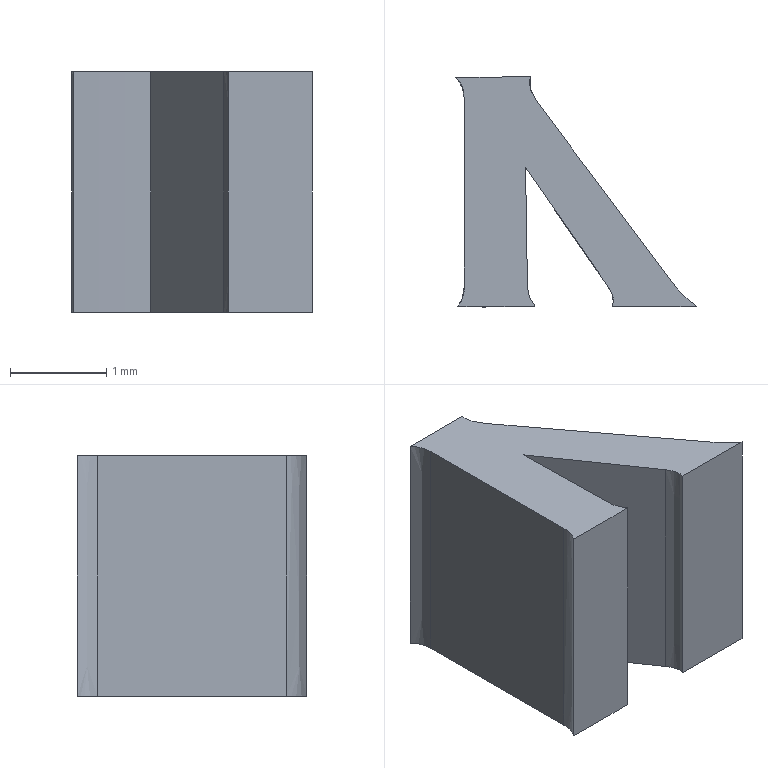Part | STEP file | lll_id1114_x_t | 1 solid | 15 faces | box 2.507 x 2.385 x 2.5 mm | volume 6.979 mm3 | plane 8 | other 4 | cylinder 3 | commonest cylinder face diameters 0.673 x1 2.106 x1 55.706 x1
STEP:
#1=CARTESIAN_POINT('',(392.49,-124.732,2.35));
#2=VERTEX_POINT('',#1);
#3=CARTESIAN_POINT('',(392.719,-124.959,2.35));
#4=VERTEX_POINT('',#3);
#5=CARTESIAN_POINT('',(393.33,-124.099,2.35));
#6=DIRECTION('',(0.,0.,1.));
#7=DIRECTION('',(-1.,0.,0.));
#8=AXIS2_PLACEMENT_3D('',#5,#6,#7);
#9=CIRCLE('',#8,1.053);
#10=EDGE_CURVE('',#2,#4,#9,.T.);
#11=ORIENTED_EDGE('',*,*,#10,.T.);
#12=CARTESIAN_POINT('',(392.719,-124.959,-0.15));
#13=VERTEX_POINT('',#12);
#14=CARTESIAN_POINT('',(392.727,-124.962,-0.15));
#15=DIRECTION('',(0.,0.,1.));
#16=VECTOR('',#15,1.);
#17=LINE('',#14,#16);
#18=EDGE_CURVE('',#13,#4,#17,.T.);
#19=ORIENTED_EDGE('',*,*,#18,.F.);
#20=CARTESIAN_POINT('',(392.49,-124.732,-0.15));
#21=VERTEX_POINT('',#20);
#22=CARTESIAN_POINT('',(393.33,-124.099,-0.15));
#23=DIRECTION('',(0.,0.,1.));
#24=DIRECTION('',(-1.,0.,0.));
#25=AXIS2_PLACEMENT_3D('',#22,#23,#24);
#26=CIRCLE('',#25,1.053);
#27=EDGE_CURVE('',#21,#13,#26,.T.);
#28=ORIENTED_EDGE('',*,*,#27,.F.);
#29=CARTESIAN_POINT('',(392.49,-124.732,-0.15));
#30=DIRECTION('',(0.,0.,1.));
#31=VECTOR('',#30,1.);
#32=LINE('',#29,#31);
#33=EDGE_CURVE('',#21,#2,#32,.T.);
#34=ORIENTED_EDGE('',*,*,#33,.T.);
#35=EDGE_LOOP('',(#11,#19,#28,#34));
#36=FACE_OUTER_BOUND('',#35,.T.);
#37=CARTESIAN_POINT('',(393.33,-124.099,-0.15));
#38=DIRECTION('',(0.,0.,1.));
#39=DIRECTION('',(1.,0.,0.));
#40=AXIS2_PLACEMENT_3D('',#37,#38,#39);
#41=CYLINDRICAL_SURFACE('',#40,1.053);
#42=ADVANCED_FACE('',(#36),#41,.F.);
#43=CARTESIAN_POINT('',(391.85,-124.96,2.35));
#44=VERTEX_POINT('',#43);
#45=CARTESIAN_POINT('',(392.719,-124.962,2.35));
#46=DIRECTION('',(-1.,0.,0.));
#47=VECTOR('',#46,1.);
#48=LINE('',#45,#47);
#49=EDGE_CURVE('',#4,#44,#48,.T.);
#50=ORIENTED_EDGE('',*,*,#49,.T.);
#51=CARTESIAN_POINT('',(391.85,-124.96,-0.15));
#52=VERTEX_POINT('',#51);
#53=CARTESIAN_POINT('',(391.849,-124.962,-0.15));
#54=DIRECTION('',(0.,0.,1.));
#55=VECTOR('',#54,1.);
#56=LINE('',#53,#55);
#57=EDGE_CURVE('',#52,#44,#56,.T.);
#58=ORIENTED_EDGE('',*,*,#57,.F.);
#59=CARTESIAN_POINT('',(392.719,-124.962,-0.15));
#60=DIRECTION('',(-1.,0.,0.));
#61=VECTOR('',#60,1.);
#62=LINE('',#59,#61);
#63=EDGE_CURVE('',#13,#52,#62,.T.);
#64=ORIENTED_EDGE('',*,*,#63,.F.);
#65=ORIENTED_EDGE('',*,*,#18,.T.);
#66=EDGE_LOOP('',(#50,#58,#64,#65));
#67=FACE_OUTER_BOUND('',#66,.T.);
#68=CARTESIAN_POINT('',(392.719,-124.962,-0.15));
#69=DIRECTION('',(0.,1.,0.));
#70=DIRECTION('',(0.,0.,1.));
#71=AXIS2_PLACEMENT_3D('',#68,#69,#70);
#72=PLANE('',#71);
#73=ADVANCED_FACE('',(#67),#72,.F.);
#74=CARTESIAN_POINT('',(391.803,-124.75,2.35));
#75=VERTEX_POINT('',#74);
#76=CARTESIAN_POINT('',(391.85,-124.958,2.35));
#77=CARTESIAN_POINT('',(391.856,-124.941,2.35));
#78=CARTESIAN_POINT('',(391.859,-124.924,2.35));
#79=CARTESIAN_POINT('',(391.86,-124.892,2.35));
#80=CARTESIAN_POINT('',(391.859,-124.877,2.35));
#81=CARTESIAN_POINT('',(391.854,-124.853,2.35));
#82=CARTESIAN_POINT('',(391.851,-124.844,2.35));
#83=CARTESIAN_POINT('',(391.844,-124.824,2.35));
#84=CARTESIAN_POINT('',(391.84,-124.814,2.35));
#85=CARTESIAN_POINT('',(391.827,-124.789,2.35));
#86=CARTESIAN_POINT('',(391.819,-124.775,2.35));
#87=CARTESIAN_POINT('',(391.808,-124.757,2.35));
#88=CARTESIAN_POINT('',(391.805,-124.753,2.35));
#89=CARTESIAN_POINT('',(391.803,-124.75,2.35));
#90=(BOUNDED_CURVE()B_SPLINE_CURVE(3,(#76,#77,#78,#79,#80,#81,#82,#83,#84,#85,#86,#87,#88,#89),.UNSPECIFIED.,.F.,.F.)B_SPLINE_CURVE_WITH_KNOTS((4,2,2,2,2,2,4),(0.,0.2364,0.4388,0.5636,0.7197,0.9376,1.),.UNSPECIFIED.)CURVE()GEOMETRIC_REPRESENTATION_ITEM()RATIONAL_B_SPLINE_CURVE((0.502,0.4993,0.4993,0.499,0.499,0.5013,0.5013,0.5014,0.5014,0.5014,0.5014,0.502,0.502,0.502))REPRESENTATION_ITEM(''));
#91=EDGE_CURVE('',#44,#75,#90,.T.);
#92=ORIENTED_EDGE('',*,*,#91,.T.);
#93=CARTESIAN_POINT('',(391.803,-124.75,-0.15));
#94=VERTEX_POINT('',#93);
#95=CARTESIAN_POINT('',(391.803,-124.75,-0.15));
#96=DIRECTION('',(0.,0.,1.));
#97=VECTOR('',#96,1.);
#98=LINE('',#95,#97);
#99=EDGE_CURVE('',#94,#75,#98,.T.);
#100=ORIENTED_EDGE('',*,*,#99,.F.);
#101=CARTESIAN_POINT('',(391.85,-124.96,-0.15));
#102=CARTESIAN_POINT('',(391.85,-124.959,-0.15));
#103=CARTESIAN_POINT('',(391.85,-124.958,-0.15));
#104=CARTESIAN_POINT('',(391.856,-124.941,-0.15));
#105=CARTESIAN_POINT('',(391.859,-124.924,-0.15));
#106=CARTESIAN_POINT('',(391.86,-124.892,-0.15));
#107=CARTESIAN_POINT('',(391.859,-124.877,-0.15));
#108=CARTESIAN_POINT('',(391.854,-124.853,-0.15));
#109=CARTESIAN_POINT('',(391.851,-124.844,-0.15));
#110=CARTESIAN_POINT('',(391.844,-124.824,-0.15));
#111=CARTESIAN_POINT('',(391.84,-124.814,-0.15));
#112=CARTESIAN_POINT('',(391.827,-124.789,-0.15));
#113=CARTESIAN_POINT('',(391.819,-124.775,-0.15));
#114=CARTESIAN_POINT('',(391.808,-124.757,-0.15));
#115=CARTESIAN_POINT('',(391.805,-124.753,-0.15));
#116=CARTESIAN_POINT('',(391.803,-124.75,-0.15));
#117=(BOUNDED_CURVE()B_SPLINE_CURVE(3,(#101,#102,#103,#104,#105,#106,#107,#108,#109,#110,#111,#112,#113,#114,#115,#116),.UNSPECIFIED.,.F.,.F.)B_SPLINE_CURVE_WITH_KNOTS((4,2,2,2,2,2,2,4),(0.,0.009901,0.2439,0.4443,0.5679,0.7225,0.9382,1.),.UNSPECIFIED.)CURVE()GEOMETRIC_REPRESENTATION_ITEM()RATIONAL_B_SPLINE_CURVE((0.502,0.502,0.502,0.4993,0.4993,0.499,0.499,0.5013,0.5013,0.5014,0.5014,0.5014,0.5014,0.502,0.502,0.502))REPRESENTATION_ITEM(''));
#118=EDGE_CURVE('',#52,#94,#117,.T.);
#119=ORIENTED_EDGE('',*,*,#118,.F.);
#120=ORIENTED_EDGE('',*,*,#57,.T.);
#121=EDGE_LOOP('',(#92,#100,#119,#120));
#122=FACE_OUTER_BOUND('',#121,.T.);
#123=CARTESIAN_POINT('',(391.849,-124.962,-0.15));
#124=CARTESIAN_POINT('',(391.849,-124.961,-0.15));
#125=CARTESIAN_POINT('',(391.849,-124.96,-0.15));
#126=CARTESIAN_POINT('',(391.85,-124.959,-0.15));
#127=CARTESIAN_POINT('',(391.85,-124.958,-0.15));
#128=CARTESIAN_POINT('',(391.856,-124.941,-0.15));
#129=CARTESIAN_POINT('',(391.859,-124.924,-0.15));
#130=CARTESIAN_POINT('',(391.86,-124.892,-0.15));
#131=CARTESIAN_POINT('',(391.859,-124.877,-0.15));
#132=CARTESIAN_POINT('',(391.854,-124.853,-0.15));
#133=CARTESIAN_POINT('',(391.851,-124.844,-0.15));
#134=CARTESIAN_POINT('',(391.844,-124.824,-0.15));
#135=CARTESIAN_POINT('',(391.84,-124.814,-0.15));
#136=CARTESIAN_POINT('',(391.827,-124.789,-0.15));
#137=CARTESIAN_POINT('',(391.819,-124.775,-0.15));
#138=CARTESIAN_POINT('',(391.808,-124.757,-0.15));
#139=CARTESIAN_POINT('',(391.805,-124.753,-0.15));
#140=CARTESIAN_POINT('',(391.803,-124.75,-0.15));
#141=(BOUNDED_CURVE()B_SPLINE_CURVE(3,(#123,#124,#125,#126,#127,#128,#129,#130,#131,#132,#133,#134,#135,#136,#137,#138,#139,#140),.UNSPECIFIED.,.F.,.F.)B_SPLINE_CURVE_WITH_KNOTS((4,2,2,2,2,2,2,2,4),(0.,0.009901,0.0197,0.2514,0.4498,0.5722,0.7252,0.9388,1.),.UNSPECIFIED.)CURVE()GEOMETRIC_REPRESENTATION_ITEM()RATIONAL_B_SPLINE_CURVE((0.502,0.502,0.502,0.502,0.502,0.4993,0.4993,0.499,0.499,0.5013,0.5013,0.5014,0.5014,0.5014,0.5014,0.502,0.502,0.502))REPRESENTATION_ITEM(''));
#142=DIRECTION('',(0.,0.,1.));
#143=VECTOR('',#142,1.);
#144=SURFACE_OF_LINEAR_EXTRUSION('',#141,#143);
#145=ADVANCED_FACE('',(#122),#144,.F.);
#146=CARTESIAN_POINT('',(390.949,-123.517,2.35));
#147=VERTEX_POINT('',#146);
#148=CARTESIAN_POINT('',(391.803,-124.75,2.35));
#149=DIRECTION('',(-0.5693,0.8221,0.));
#150=VECTOR('',#149,1.);
#151=LINE('',#148,#150);
#152=EDGE_CURVE('',#75,#147,#151,.T.);
#153=ORIENTED_EDGE('',*,*,#152,.T.);
#154=CARTESIAN_POINT('',(390.949,-123.517,-0.15));
#155=VERTEX_POINT('',#154);
#156=CARTESIAN_POINT('',(390.949,-123.517,-0.15));
#157=DIRECTION('',(0.,0.,1.));
#158=VECTOR('',#157,1.);
#159=LINE('',#156,#158);
#160=EDGE_CURVE('',#155,#147,#159,.T.);
#161=ORIENTED_EDGE('',*,*,#160,.F.);
#162=CARTESIAN_POINT('',(391.803,-124.75,-0.15));
#163=DIRECTION('',(-0.5693,0.8221,0.));
#164=VECTOR('',#163,1.);
#165=LINE('',#162,#164);
#166=EDGE_CURVE('',#94,#155,#165,.T.);
#167=ORIENTED_EDGE('',*,*,#166,.F.);
#168=ORIENTED_EDGE('',*,*,#99,.T.);
#169=EDGE_LOOP('',(#153,#161,#167,#168));
#170=FACE_OUTER_BOUND('',#169,.T.);
#171=CARTESIAN_POINT('',(391.803,-124.75,-0.15));
#172=DIRECTION('',(0.8221,0.5693,0.));
#173=DIRECTION('',(0.5693,-0.8221,0.));
#174=AXIS2_PLACEMENT_3D('',#171,#172,#173);
#175=PLANE('',#174);
#176=ADVANCED_FACE('',(#170),#175,.F.);
#177=CARTESIAN_POINT('',(390.968,-124.746,2.35));
#178=VERTEX_POINT('',#177);
#179=CARTESIAN_POINT('',(390.949,-123.517,2.35));
#180=DIRECTION('',(0.01539,-0.9999,0.));
#181=VECTOR('',#180,1.);
#182=LINE('',#179,#181);
#183=EDGE_CURVE('',#147,#178,#182,.T.);
#184=ORIENTED_EDGE('',*,*,#183,.T.);
#185=CARTESIAN_POINT('',(390.968,-124.746,-0.15));
#186=VERTEX_POINT('',#185);
#187=CARTESIAN_POINT('',(390.968,-124.746,-0.15));
#188=DIRECTION('',(0.,0.,1.));
#189=VECTOR('',#188,1.);
#190=LINE('',#187,#189);
#191=EDGE_CURVE('',#186,#178,#190,.T.);
#192=ORIENTED_EDGE('',*,*,#191,.F.);
#193=CARTESIAN_POINT('',(390.949,-123.517,-0.15));
#194=DIRECTION('',(0.01539,-0.9999,0.));
#195=VECTOR('',#194,1.);
#196=LINE('',#193,#195);
#197=EDGE_CURVE('',#155,#186,#196,.T.);
#198=ORIENTED_EDGE('',*,*,#197,.F.);
#199=ORIENTED_EDGE('',*,*,#160,.T.);
#200=EDGE_LOOP('',(#184,#192,#198,#199));
#201=FACE_OUTER_BOUND('',#200,.T.);
#202=CARTESIAN_POINT('',(390.949,-123.517,-0.15));
#203=DIRECTION('',(-0.9999,-0.01539,0.));
#204=DIRECTION('',(-0.01539,0.9999,0.));
#205=AXIS2_PLACEMENT_3D('',#202,#203,#204);
#206=PLANE('',#205);
#207=ADVANCED_FACE('',(#201),#206,.F.);
#208=CARTESIAN_POINT('',(391.045,-124.956,2.35));
#209=VERTEX_POINT('',#208);
#210=CARTESIAN_POINT('',(391.305,-124.743,2.35));
#211=DIRECTION('',(0.,0.,1.));
#212=DIRECTION('',(-1.,0.,0.));
#213=AXIS2_PLACEMENT_3D('',#210,#211,#212);
#214=CIRCLE('',#213,0.3365);
#215=EDGE_CURVE('',#178,#209,#214,.T.);
#216=ORIENTED_EDGE('',*,*,#215,.T.);
#217=CARTESIAN_POINT('',(391.045,-124.956,-0.15));
#218=VERTEX_POINT('',#217);
#219=CARTESIAN_POINT('',(391.045,-124.956,-0.15));
#220=DIRECTION('',(0.,0.,1.));
#221=VECTOR('',#220,1.);
#222=LINE('',#219,#221);
#223=EDGE_CURVE('',#218,#209,#222,.T.);
#224=ORIENTED_EDGE('',*,*,#223,.F.);
#225=CARTESIAN_POINT('',(391.305,-124.743,-0.15));
#226=DIRECTION('',(0.,0.,1.));
#227=DIRECTION('',(-1.,0.,0.));
#228=AXIS2_PLACEMENT_3D('',#225,#226,#227);
#229=CIRCLE('',#228,0.3365);
#230=EDGE_CURVE('',#186,#218,#229,.T.);
#231=ORIENTED_EDGE('',*,*,#230,.F.);
#232=ORIENTED_EDGE('',*,*,#191,.T.);
#233=EDGE_LOOP('',(#216,#224,#231,#232));
#234=FACE_OUTER_BOUND('',#233,.T.);
#235=CARTESIAN_POINT('',(391.305,-124.743,-0.15));
#236=DIRECTION('',(0.,0.,1.));
#237=DIRECTION('',(1.,0.,0.));
#238=AXIS2_PLACEMENT_3D('',#235,#236,#237);
#239=CYLINDRICAL_SURFACE('',#238,0.3365);
#240=ADVANCED_FACE('',(#234),#239,.F.);
#241=CARTESIAN_POINT('',(390.246,-124.959,2.35));
#242=VERTEX_POINT('',#241);
#243=CARTESIAN_POINT('',(390.459,-97.11,2.35));
#244=DIRECTION('',(0.,0.,-1.));
#245=DIRECTION('',(-1.,0.,0.));
#246=AXIS2_PLACEMENT_3D('',#243,#244,#245);
#247=CIRCLE('',#246,27.853);
#248=EDGE_CURVE('',#209,#242,#247,.T.);
#249=ORIENTED_EDGE('',*,*,#248,.T.);
#250=CARTESIAN_POINT('',(390.246,-124.959,-0.15));
#251=VERTEX_POINT('',#250);
#252=CARTESIAN_POINT('',(390.239,-124.962,-0.15));
#253=DIRECTION('',(0.,0.,1.));
#254=VECTOR('',#253,1.);
#255=LINE('',#252,#254);
#256=EDGE_CURVE('',#251,#242,#255,.T.);
#257=ORIENTED_EDGE('',*,*,#256,.F.);
#258=CARTESIAN_POINT('',(390.459,-97.11,-0.15));
#259=DIRECTION('',(0.,0.,-1.));
#260=DIRECTION('',(-1.,0.,0.));
#261=AXIS2_PLACEMENT_3D('',#258,#259,#260);
#262=CIRCLE('',#261,27.853);
#263=EDGE_CURVE('',#218,#251,#262,.T.);
#264=ORIENTED_EDGE('',*,*,#263,.F.);
#265=ORIENTED_EDGE('',*,*,#223,.T.);
#266=EDGE_LOOP('',(#249,#257,#264,#265));
#267=FACE_OUTER_BOUND('',#266,.T.);
#268=CARTESIAN_POINT('',(390.459,-97.11,-0.15));
#269=DIRECTION('',(0.,0.,1.));
#270=DIRECTION('',(1.,0.,0.));
#271=AXIS2_PLACEMENT_3D('',#268,#269,#270);
#272=CYLINDRICAL_SURFACE('',#271,27.853);
#273=ADVANCED_FACE('',(#267),#272,.T.);
#274=CARTESIAN_POINT('',(390.314,-124.75,2.35));
#275=VERTEX_POINT('',#274);
#276=CARTESIAN_POINT('',(390.244,-124.956,2.35));
#277=CARTESIAN_POINT('',(390.252,-124.948,2.35));
#278=CARTESIAN_POINT('',(390.26,-124.939,2.35));
#279=CARTESIAN_POINT('',(390.276,-124.916,2.35));
#280=CARTESIAN_POINT('',(390.284,-124.902,2.35));
#281=CARTESIAN_POINT('',(390.296,-124.874,2.35));
#282=CARTESIAN_POINT('',(390.3,-124.86,2.35));
#283=CARTESIAN_POINT('',(390.307,-124.833,2.35));
#284=CARTESIAN_POINT('',(390.309,-124.819,2.35));
#285=CARTESIAN_POINT('',(390.313,-124.789,2.35));
#286=CARTESIAN_POINT('',(390.314,-124.773,2.35));
#287=CARTESIAN_POINT('',(390.314,-124.754,2.35));
#288=CARTESIAN_POINT('',(390.314,-124.752,2.35));
#289=CARTESIAN_POINT('',(390.314,-124.75,2.35));
#290=(BOUNDED_CURVE()B_SPLINE_CURVE(3,(#276,#277,#278,#279,#280,#281,#282,#283,#284,#285,#286,#287,#288,#289),.UNSPECIFIED.,.F.,.F.)B_SPLINE_CURVE_WITH_KNOTS((4,2,2,2,2,2,4),(0.,0.1579,0.3766,0.5639,0.7508,0.9688,1.),.UNSPECIFIED.)CURVE()GEOMETRIC_REPRESENTATION_ITEM()RATIONAL_B_SPLINE_CURVE((0.5005,0.4998,0.4998,0.4984,0.4984,0.4995,0.4995,0.4999,0.4999,0.5001,0.5001,0.5005,0.5005,0.5005))REPRESENTATION_ITEM(''));
#291=EDGE_CURVE('',#242,#275,#290,.T.);
#292=ORIENTED_EDGE('',*,*,#291,.T.);
#293=CARTESIAN_POINT('',(390.314,-124.75,-0.15));
#294=VERTEX_POINT('',#293);
#295=CARTESIAN_POINT('',(390.314,-124.75,-0.15));
#296=DIRECTION('',(0.,0.,1.));
#297=VECTOR('',#296,1.);
#298=LINE('',#295,#297);
#299=EDGE_CURVE('',#294,#275,#298,.T.);
#300=ORIENTED_EDGE('',*,*,#299,.F.);
#301=CARTESIAN_POINT('',(390.243,-124.958,-0.15));
#302=CARTESIAN_POINT('',(390.243,-124.957,-0.15));
#303=CARTESIAN_POINT('',(390.244,-124.957,-0.15));
#304=CARTESIAN_POINT('',(390.252,-124.948,-0.15));
#305=CARTESIAN_POINT('',(390.26,-124.939,-0.15));
#306=CARTESIAN_POINT('',(390.276,-124.916,-0.15));
#307=CARTESIAN_POINT('',(390.284,-124.902,-0.15));
#308=CARTESIAN_POINT('',(390.296,-124.874,-0.15));
#309=CARTESIAN_POINT('',(390.3,-124.86,-0.15));
#310=CARTESIAN_POINT('',(390.307,-124.833,-0.15));
#311=CARTESIAN_POINT('',(390.309,-124.819,-0.15));
#312=CARTESIAN_POINT('',(390.313,-124.789,-0.15));
#313=CARTESIAN_POINT('',(390.314,-124.773,-0.15));
#314=CARTESIAN_POINT('',(390.314,-124.754,-0.15));
#315=CARTESIAN_POINT('',(390.314,-124.752,-0.15));
#316=CARTESIAN_POINT('',(390.314,-124.75,-0.15));
#317=(BOUNDED_CURVE()B_SPLINE_CURVE(3,(#301,#302,#303,#304,#305,#306,#307,#308,#309,#310,#311,#312,#313,#314,#315,#316),.UNSPECIFIED.,.F.,.F.)B_SPLINE_CURVE_WITH_KNOTS((4,2,2,2,2,2,2,4),(0.,0.009901,0.1662,0.3828,0.5682,0.7532,0.9691,1.),.UNSPECIFIED.)CURVE()GEOMETRIC_REPRESENTATION_ITEM()RATIONAL_B_SPLINE_CURVE((0.5005,0.5005,0.5005,0.4998,0.4998,0.4984,0.4984,0.4995,0.4995,0.4999,0.4999,0.5001,0.5001,0.5005,0.5005,0.5005))REPRESENTATION_ITEM(''));
#318=EDGE_CURVE('',#251,#294,#317,.T.);
#319=ORIENTED_EDGE('',*,*,#318,.F.);
#320=ORIENTED_EDGE('',*,*,#256,.T.);
#321=EDGE_LOOP('',(#292,#300,#319,#320));
#322=FACE_OUTER_BOUND('',#321,.T.);
#323=CARTESIAN_POINT('',(390.239,-124.962,-0.15));
#324=CARTESIAN_POINT('',(390.24,-124.96,-0.15));
#325=CARTESIAN_POINT('',(390.242,-124.959,-0.15));
#326=CARTESIAN_POINT('',(390.243,-124.957,-0.15));
#327=CARTESIAN_POINT('',(390.244,-124.957,-0.15));
#328=CARTESIAN_POINT('',(390.252,-124.948,-0.15));
#329=CARTESIAN_POINT('',(390.26,-124.939,-0.15));
#330=CARTESIAN_POINT('',(390.276,-124.916,-0.15));
#331=CARTESIAN_POINT('',(390.284,-124.902,-0.15));
#332=CARTESIAN_POINT('',(390.296,-124.874,-0.15));
#333=CARTESIAN_POINT('',(390.3,-124.86,-0.15));
#334=CARTESIAN_POINT('',(390.307,-124.833,-0.15));
#335=CARTESIAN_POINT('',(390.309,-124.819,-0.15));
#336=CARTESIAN_POINT('',(390.313,-124.789,-0.15));
#337=CARTESIAN_POINT('',(390.314,-124.773,-0.15));
#338=CARTESIAN_POINT('',(390.314,-124.754,-0.15));
#339=CARTESIAN_POINT('',(390.314,-124.752,-0.15));
#340=CARTESIAN_POINT('',(390.314,-124.75,-0.15));
#341=(BOUNDED_CURVE()B_SPLINE_CURVE(3,(#323,#324,#325,#326,#327,#328,#329,#330,#331,#332,#333,#334,#335,#336,#337,#338,#339,#340),.UNSPECIFIED.,.F.,.F.)B_SPLINE_CURVE_WITH_KNOTS((4,2,2,2,2,2,2,2,4),(0.,0.02341,0.03308,0.1858,0.3972,0.5784,0.759,0.9698,1.),.UNSPECIFIED.)CURVE()GEOMETRIC_REPRESENTATION_ITEM()RATIONAL_B_SPLINE_CURVE((0.5005,0.5005,0.5005,0.5005,0.5005,0.4998,0.4998,0.4984,0.4984,0.4995,0.4995,0.4999,0.4999,0.5001,0.5001,0.5005,0.5005,0.5005))REPRESENTATION_ITEM(''));
#342=DIRECTION('',(0.,0.,1.));
#343=VECTOR('',#342,1.);
#344=SURFACE_OF_LINEAR_EXTRUSION('',#341,#343);
#345=ADVANCED_FACE('',(#322),#344,.F.);
#346=CARTESIAN_POINT('',(390.311,-122.789,2.35));
#347=VERTEX_POINT('',#346);
#348=CARTESIAN_POINT('',(390.314,-124.75,2.35));
#349=DIRECTION('',(-0.00155,1.,0.));
#350=VECTOR('',#349,1.);
#351=LINE('',#348,#350);
#352=EDGE_CURVE('',#275,#347,#351,.T.);
#353=ORIENTED_EDGE('',*,*,#352,.T.);
#354=CARTESIAN_POINT('',(390.311,-122.789,-0.15));
#355=VERTEX_POINT('',#354);
#356=CARTESIAN_POINT('',(390.311,-122.789,-0.15));
#357=DIRECTION('',(0.,0.,1.));
#358=VECTOR('',#357,1.);
#359=LINE('',#356,#358);
#360=EDGE_CURVE('',#355,#347,#359,.T.);
#361=ORIENTED_EDGE('',*,*,#360,.F.);
#362=CARTESIAN_POINT('',(390.314,-124.75,-0.15));
#363=DIRECTION('',(-0.00155,1.,0.));
#364=VECTOR('',#363,1.);
#365=LINE('',#362,#364);
#366=EDGE_CURVE('',#294,#355,#365,.T.);
#367=ORIENTED_EDGE('',*,*,#366,.F.);
#368=ORIENTED_EDGE('',*,*,#299,.T.);
#369=EDGE_LOOP('',(#353,#361,#367,#368));
#370=FACE_OUTER_BOUND('',#369,.T.);
#371=CARTESIAN_POINT('',(390.314,-124.75,-0.15));
#372=DIRECTION('',(1.,0.00155,0.));
#373=DIRECTION('',(0.00155,-1.,0.));
#374=AXIS2_PLACEMENT_3D('',#371,#372,#373);
#375=PLANE('',#374);
#376=ADVANCED_FACE('',(#370),#375,.F.);
#377=CARTESIAN_POINT('',(390.226,-122.58,2.35));
#378=VERTEX_POINT('',#377);
#379=CARTESIAN_POINT('',(390.311,-122.789,2.35));
#380=CARTESIAN_POINT('',(390.311,-122.768,2.35));
#381=CARTESIAN_POINT('',(390.309,-122.746,2.35));
#382=CARTESIAN_POINT('',(390.302,-122.711,2.35));
#383=CARTESIAN_POINT('',(390.298,-122.697,2.35));
#384=CARTESIAN_POINT('',(390.285,-122.658,2.35));
#385=CARTESIAN_POINT('',(390.272,-122.635,2.35));
#386=CARTESIAN_POINT('',(390.248,-122.604,2.35));
#387=CARTESIAN_POINT('',(390.24,-122.596,2.35));
#388=CARTESIAN_POINT('',(390.229,-122.586,2.35));
#389=CARTESIAN_POINT('',(390.227,-122.584,2.35));
#390=CARTESIAN_POINT('',(390.226,-122.583,2.35));
#391=(BOUNDED_CURVE()B_SPLINE_CURVE(3,(#379,#380,#381,#382,#383,#384,#385,#386,#387,#388,#389,#390),.UNSPECIFIED.,.F.,.F.)B_SPLINE_CURVE_WITH_KNOTS((4,2,2,2,2,4),(0.,0.2827,0.4704,0.8135,0.969,1.),.UNSPECIFIED.)CURVE()GEOMETRIC_REPRESENTATION_ITEM()RATIONAL_B_SPLINE_CURVE((0.5011,0.4996,0.4996,0.5001,0.5001,0.4961,0.4961,0.5002,0.5002,0.501,0.501,0.5011))REPRESENTATION_ITEM(''));
#392=EDGE_CURVE('',#347,#378,#391,.T.);
#393=ORIENTED_EDGE('',*,*,#392,.T.);
#394=CARTESIAN_POINT('',(390.226,-122.58,-0.15));
#395=VERTEX_POINT('',#394);
#396=CARTESIAN_POINT('',(390.22,-122.578,-0.15));
#397=DIRECTION('',(0.,0.,1.));
#398=VECTOR('',#397,1.);
#399=LINE('',#396,#398);
#400=EDGE_CURVE('',#395,#378,#399,.T.);
#401=ORIENTED_EDGE('',*,*,#400,.F.);
#402=CARTESIAN_POINT('',(390.311,-122.789,-0.15));
#403=CARTESIAN_POINT('',(390.311,-122.768,-0.15));
#404=CARTESIAN_POINT('',(390.309,-122.746,-0.15));
#405=CARTESIAN_POINT('',(390.302,-122.711,-0.15));
#406=CARTESIAN_POINT('',(390.298,-122.697,-0.15));
#407=CARTESIAN_POINT('',(390.285,-122.658,-0.15));
#408=CARTESIAN_POINT('',(390.272,-122.635,-0.15));
#409=CARTESIAN_POINT('',(390.248,-122.604,-0.15));
#410=CARTESIAN_POINT('',(390.24,-122.596,-0.15));
#411=CARTESIAN_POINT('',(390.229,-122.586,-0.15));
#412=CARTESIAN_POINT('',(390.227,-122.584,-0.15));
#413=CARTESIAN_POINT('',(390.225,-122.582,-0.15));
#414=CARTESIAN_POINT('',(390.225,-122.582,-0.15));
#415=CARTESIAN_POINT('',(390.224,-122.581,-0.15));
#416=(BOUNDED_CURVE()B_SPLINE_CURVE(3,(#402,#403,#404,#405,#406,#407,#408,#409,#410,#411,#412,#413,#414,#415),.UNSPECIFIED.,.F.,.F.)B_SPLINE_CURVE_WITH_KNOTS((4,2,2,2,2,2,4),(0.,0.2799,0.4657,0.8054,0.9594,0.9901,1.),.UNSPECIFIED.)CURVE()GEOMETRIC_REPRESENTATION_ITEM()RATIONAL_B_SPLINE_CURVE((0.5011,0.4996,0.4996,0.5001,0.5001,0.4961,0.4961,0.5002,0.5002,0.501,0.501,0.5011,0.5011,0.5011))REPRESENTATION_ITEM(''));
#417=EDGE_CURVE('',#355,#395,#416,.T.);
#418=ORIENTED_EDGE('',*,*,#417,.F.);
#419=ORIENTED_EDGE('',*,*,#360,.T.);
#420=EDGE_LOOP('',(#393,#401,#418,#419));
#421=FACE_OUTER_BOUND('',#420,.T.);
#422=CARTESIAN_POINT('',(390.311,-122.789,-0.15));
#423=CARTESIAN_POINT('',(390.311,-122.768,-0.15));
#424=CARTESIAN_POINT('',(390.309,-122.746,-0.15));
#425=CARTESIAN_POINT('',(390.302,-122.711,-0.15));
#426=CARTESIAN_POINT('',(390.298,-122.697,-0.15));
#427=CARTESIAN_POINT('',(390.285,-122.658,-0.15));
#428=CARTESIAN_POINT('',(390.272,-122.635,-0.15));
#429=CARTESIAN_POINT('',(390.248,-122.604,-0.15));
#430=CARTESIAN_POINT('',(390.24,-122.596,-0.15));
#431=CARTESIAN_POINT('',(390.229,-122.586,-0.15));
#432=CARTESIAN_POINT('',(390.227,-122.584,-0.15));
#433=CARTESIAN_POINT('',(390.225,-122.582,-0.15));
#434=CARTESIAN_POINT('',(390.225,-122.582,-0.15));
#435=CARTESIAN_POINT('',(390.223,-122.58,-0.15));
#436=CARTESIAN_POINT('',(390.223,-122.58,-0.15));
#437=CARTESIAN_POINT('',(390.222,-122.579,-0.15));
#438=CARTESIAN_POINT('',(390.221,-122.578,-0.15));
#439=CARTESIAN_POINT('',(390.22,-122.578,-0.15));
#440=(BOUNDED_CURVE()B_SPLINE_CURVE(3,(#422,#423,#424,#425,#426,#427,#428,#429,#430,#431,#432,#433,#434,#435,#436,#437,#438,#439),.UNSPECIFIED.,.F.,.F.)B_SPLINE_CURVE_WITH_KNOTS((4,2,2,2,2,2,2,2,4),(0.,0.2743,0.4563,0.7891,0.9399,0.9701,0.9798,0.9896,1.),.UNSPECIFIED.)CURVE()GEOMETRIC_REPRESENTATION_ITEM()RATIONAL_B_SPLINE_CURVE((0.5011,0.4996,0.4996,0.5001,0.5001,0.4961,0.4961,0.5002,0.5002,0.501,0.501,0.5011,0.5011,0.5011,0.5011,0.5011,0.5011,0.5011))REPRESENTATION_ITEM(''));
#441=DIRECTION('',(0.,0.,1.));
#442=VECTOR('',#441,1.);
#443=SURFACE_OF_LINEAR_EXTRUSION('',#440,#442);
#444=ADVANCED_FACE('',(#421),#443,.F.);
#445=CARTESIAN_POINT('',(390.998,-122.58,2.35));
#446=VERTEX_POINT('',#445);
#447=CARTESIAN_POINT('',(390.226,-122.578,2.35));
#448=DIRECTION('',(1.,0.,0.));
#449=VECTOR('',#448,1.);
#450=LINE('',#447,#449);
#451=EDGE_CURVE('',#378,#446,#450,.T.);
#452=ORIENTED_EDGE('',*,*,#451,.T.);
#453=CARTESIAN_POINT('',(390.998,-122.58,-0.15));
#454=VERTEX_POINT('',#453);
#455=CARTESIAN_POINT('',(391.,-122.578,-0.15));
#456=DIRECTION('',(0.,0.,1.));
#457=VECTOR('',#456,1.);
#458=LINE('',#455,#457);
#459=EDGE_CURVE('',#454,#446,#458,.T.);
#460=ORIENTED_EDGE('',*,*,#459,.F.);
#461=CARTESIAN_POINT('',(390.226,-122.578,-0.15));
#462=DIRECTION('',(1.,0.,0.));
#463=VECTOR('',#462,1.);
#464=LINE('',#461,#463);
#465=EDGE_CURVE('',#395,#454,#464,.T.);
#466=ORIENTED_EDGE('',*,*,#465,.F.);
#467=ORIENTED_EDGE('',*,*,#400,.T.);
#468=EDGE_LOOP('',(#452,#460,#466,#467));
#469=FACE_OUTER_BOUND('',#468,.T.);
#470=CARTESIAN_POINT('',(390.226,-122.578,-0.15));
#471=DIRECTION('',(0.,-1.,0.));
#472=DIRECTION('',(0.,0.,-1.));
#473=AXIS2_PLACEMENT_3D('',#470,#471,#472);
#474=PLANE('',#473);
#475=ADVANCED_FACE('',(#469),#474,.F.);
#476=CARTESIAN_POINT('',(391.131,-122.921,2.35));
#477=VERTEX_POINT('',#476);
#478=CARTESIAN_POINT('',(390.998,-122.582,2.35));
#479=CARTESIAN_POINT('',(390.997,-122.586,2.35));
#480=CARTESIAN_POINT('',(390.996,-122.589,2.35));
#481=CARTESIAN_POINT('',(390.987,-122.624,2.35));
#482=CARTESIAN_POINT('',(390.988,-122.656,2.35));
#483=CARTESIAN_POINT('',(391.,-122.704,2.35));
#484=CARTESIAN_POINT('',(391.006,-122.721,2.35));
#485=CARTESIAN_POINT('',(391.017,-122.746,2.35));
#486=CARTESIAN_POINT('',(391.021,-122.755,2.35));
#487=CARTESIAN_POINT('',(391.032,-122.774,2.35));
#488=CARTESIAN_POINT('',(391.038,-122.784,2.35));
#489=CARTESIAN_POINT('',(391.05,-122.804,2.35));
#490=CARTESIAN_POINT('',(391.057,-122.814,2.35));
#491=CARTESIAN_POINT('',(391.076,-122.844,2.35));
#492=CARTESIAN_POINT('',(391.09,-122.864,2.35));
#493=CARTESIAN_POINT('',(391.112,-122.896,2.35));
#494=CARTESIAN_POINT('',(391.122,-122.909,2.35));
#495=CARTESIAN_POINT('',(391.131,-122.921,2.35));
#496=(BOUNDED_CURVE()B_SPLINE_CURVE(3,(#478,#479,#480,#481,#482,#483,#484,#485,#486,#487,#488,#489,#490,#491,#492,#493,#494,#495),.UNSPECIFIED.,.F.,.F.)B_SPLINE_CURVE_WITH_KNOTS((4,2,2,2,2,2,2,2,4),(0.,0.03202,0.2839,0.4243,0.5019,0.5952,0.6887,0.8755,1.),.UNSPECIFIED.)CURVE()GEOMETRIC_REPRESENTATION_ITEM()RATIONAL_B_SPLINE_CURVE((0.5001,0.5,0.5,0.4903,0.4903,0.4986,0.4986,0.4998,0.4998,0.4999,0.4999,0.5,0.5,0.5,0.5,0.5,0.5,0.5001))REPRESENTATION_ITEM(''));
#497=EDGE_CURVE('',#446,#477,#496,.T.);
#498=ORIENTED_EDGE('',*,*,#497,.T.);
#499=CARTESIAN_POINT('',(391.131,-122.921,-0.15));
#500=VERTEX_POINT('',#499);
#501=CARTESIAN_POINT('',(391.131,-122.921,-0.15));
#502=DIRECTION('',(0.,0.,1.));
#503=VECTOR('',#502,1.);
#504=LINE('',#501,#503);
#505=EDGE_CURVE('',#500,#477,#504,.T.);
#506=ORIENTED_EDGE('',*,*,#505,.F.);
#507=CARTESIAN_POINT('',(390.999,-122.578,-0.15));
#508=CARTESIAN_POINT('',(390.999,-122.579,-0.15));
#509=CARTESIAN_POINT('',(390.999,-122.581,-0.15));
#510=CARTESIAN_POINT('',(390.997,-122.586,-0.15));
#511=CARTESIAN_POINT('',(390.996,-122.589,-0.15));
#512=CARTESIAN_POINT('',(390.987,-122.624,-0.15));
#513=CARTESIAN_POINT('',(390.988,-122.656,-0.15));
#514=CARTESIAN_POINT('',(391.,-122.704,-0.15));
#515=CARTESIAN_POINT('',(391.006,-122.721,-0.15));
#516=CARTESIAN_POINT('',(391.017,-122.746,-0.15));
#517=CARTESIAN_POINT('',(391.021,-122.755,-0.15));
#518=CARTESIAN_POINT('',(391.032,-122.774,-0.15));
#519=CARTESIAN_POINT('',(391.038,-122.784,-0.15));
#520=CARTESIAN_POINT('',(391.05,-122.804,-0.15));
#521=CARTESIAN_POINT('',(391.057,-122.814,-0.15));
#522=CARTESIAN_POINT('',(391.076,-122.844,-0.15));
#523=CARTESIAN_POINT('',(391.09,-122.864,-0.15));
#524=CARTESIAN_POINT('',(391.112,-122.896,-0.15));
#525=CARTESIAN_POINT('',(391.122,-122.909,-0.15));
#526=CARTESIAN_POINT('',(391.131,-122.921,-0.15));
#527=(BOUNDED_CURVE()B_SPLINE_CURVE(3,(#507,#508,#509,#510,#511,#512,#513,#514,#515,#516,#517,#518,#519,#520,#521,#522,#523,#524,#525,#526),.UNSPECIFIED.,.F.,.F.)B_SPLINE_CURVE_WITH_KNOTS((4,2,2,2,2,2,2,2,2,4),(0.,0.009901,0.0416,0.291,0.43,0.5068,0.5993,0.6918,0.8767,1.),.UNSPECIFIED.)CURVE()GEOMETRIC_REPRESENTATION_ITEM()RATIONAL_B_SPLINE_CURVE((0.5001,0.5001,0.5001,0.5,0.5,0.4903,0.4903,0.4986,0.4986,0.4998,0.4998,0.4999,0.4999,0.5,0.5,0.5,0.5,0.5,0.5,0.5001))REPRESENTATION_ITEM(''));
#528=EDGE_CURVE('',#454,#500,#527,.T.);
#529=ORIENTED_EDGE('',*,*,#528,.F.);
#530=ORIENTED_EDGE('',*,*,#459,.T.);
#531=EDGE_LOOP('',(#498,#506,#529,#530));
#532=FACE_OUTER_BOUND('',#531,.T.);
#533=CARTESIAN_POINT('',(391.,-122.575,-0.15));
#534=CARTESIAN_POINT('',(391.,-122.576,-0.15));
#535=CARTESIAN_POINT('',(391.,-122.577,-0.15));
#536=CARTESIAN_POINT('',(390.999,-122.579,-0.15));
#537=CARTESIAN_POINT('',(390.999,-122.581,-0.15));
#538=CARTESIAN_POINT('',(390.997,-122.586,-0.15));
#539=CARTESIAN_POINT('',(390.996,-122.589,-0.15));
#540=CARTESIAN_POINT('',(390.987,-122.624,-0.15));
#541=CARTESIAN_POINT('',(390.988,-122.656,-0.15));
#542=CARTESIAN_POINT('',(391.,-122.704,-0.15));
#543=CARTESIAN_POINT('',(391.006,-122.721,-0.15));
#544=CARTESIAN_POINT('',(391.017,-122.746,-0.15));
#545=CARTESIAN_POINT('',(391.021,-122.755,-0.15));
#546=CARTESIAN_POINT('',(391.032,-122.774,-0.15));
#547=CARTESIAN_POINT('',(391.038,-122.784,-0.15));
#548=CARTESIAN_POINT('',(391.05,-122.804,-0.15));
#549=CARTESIAN_POINT('',(391.057,-122.814,-0.15));
#550=CARTESIAN_POINT('',(391.076,-122.844,-0.15));
#551=CARTESIAN_POINT('',(391.09,-122.864,-0.15));
#552=CARTESIAN_POINT('',(391.112,-122.896,-0.15));
#553=CARTESIAN_POINT('',(391.122,-122.909,-0.15));
#554=CARTESIAN_POINT('',(391.131,-122.921,-0.15));
#555=(BOUNDED_CURVE()B_SPLINE_CURVE(3,(#533,#534,#535,#536,#537,#538,#539,#540,#541,#542,#543,#544,#545,#546,#547,#548,#549,#550,#551,#552,#553,#554),.UNSPECIFIED.,.F.,.F.)B_SPLINE_CURVE_WITH_KNOTS((4,2,2,2,2,2,2,2,2,2,4),(0.,0.009901,0.0197,0.05109,0.298,0.4356,0.5117,0.6032,0.6948,0.8779,1.),.UNSPECIFIED.)CURVE()GEOMETRIC_REPRESENTATION_ITEM()RATIONAL_B_SPLINE_CURVE((0.5001,0.5001,0.5001,0.5001,0.5001,0.5,0.5,0.4903,0.4903,0.4986,0.4986,0.4998,0.4998,0.4999,0.4999,0.5,0.5,0.5,0.5,0.5,0.5,0.5001))REPRESENTATION_ITEM(''));
#556=DIRECTION('',(0.,0.,1.));
#557=VECTOR('',#556,1.);
#558=SURFACE_OF_LINEAR_EXTRUSION('',#555,#557);
#559=ADVANCED_FACE('',(#532),#558,.F.);
#560=CARTESIAN_POINT('',(391.131,-122.921,2.35));
#561=DIRECTION('',(0.5999,-0.8001,0.));
#562=VECTOR('',#561,1.);
#563=LINE('',#560,#562);
#564=EDGE_CURVE('',#477,#2,#563,.T.);
#565=ORIENTED_EDGE('',*,*,#564,.T.);
#566=ORIENTED_EDGE('',*,*,#33,.F.);
#567=CARTESIAN_POINT('',(391.131,-122.921,-0.15));
#568=DIRECTION('',(0.5999,-0.8001,0.));
#569=VECTOR('',#568,1.);
#570=LINE('',#567,#569);
#571=EDGE_CURVE('',#500,#21,#570,.T.);
#572=ORIENTED_EDGE('',*,*,#571,.F.);
#573=ORIENTED_EDGE('',*,*,#505,.T.);
#574=EDGE_LOOP('',(#565,#566,#572,#573));
#575=FACE_OUTER_BOUND('',#574,.T.);
#576=CARTESIAN_POINT('',(391.131,-122.921,-0.15));
#577=DIRECTION('',(-0.8001,-0.5999,0.));
#578=DIRECTION('',(-0.5999,0.8001,0.));
#579=AXIS2_PLACEMENT_3D('',#576,#577,#578);
#580=PLANE('',#579);
#581=ADVANCED_FACE('',(#575),#580,.F.);
#582=ORIENTED_EDGE('',*,*,#27,.T.);
#583=ORIENTED_EDGE('',*,*,#63,.T.);
#584=ORIENTED_EDGE('',*,*,#118,.T.);
#585=ORIENTED_EDGE('',*,*,#166,.T.);
#586=ORIENTED_EDGE('',*,*,#197,.T.);
#587=ORIENTED_EDGE('',*,*,#230,.T.);
#588=ORIENTED_EDGE('',*,*,#263,.T.);
#589=ORIENTED_EDGE('',*,*,#318,.T.);
#590=ORIENTED_EDGE('',*,*,#366,.T.);
#591=ORIENTED_EDGE('',*,*,#417,.T.);
#592=ORIENTED_EDGE('',*,*,#465,.T.);
#593=ORIENTED_EDGE('',*,*,#528,.T.);
#594=ORIENTED_EDGE('',*,*,#571,.T.);
#595=EDGE_LOOP('',(#582,#583,#584,#585,#586,#587,#588,#589,#590,#591,#592,#593,#594));
#596=FACE_OUTER_BOUND('',#595,.T.);
#597=CARTESIAN_POINT('',(393.33,-124.099,-0.15));
#598=DIRECTION('',(0.,0.,1.));
#599=DIRECTION('',(1.,0.,0.));
#600=AXIS2_PLACEMENT_3D('',#597,#598,#599);
#601=PLANE('',#600);
#602=ADVANCED_FACE('',(#596),#601,.F.);
#603=ORIENTED_EDGE('',*,*,#10,.F.);
#604=ORIENTED_EDGE('',*,*,#564,.F.);
#605=ORIENTED_EDGE('',*,*,#497,.F.);
#606=ORIENTED_EDGE('',*,*,#451,.F.);
#607=ORIENTED_EDGE('',*,*,#392,.F.);
#608=ORIENTED_EDGE('',*,*,#352,.F.);
#609=ORIENTED_EDGE('',*,*,#291,.F.);
#610=ORIENTED_EDGE('',*,*,#248,.F.);
#611=ORIENTED_EDGE('',*,*,#215,.F.);
#612=ORIENTED_EDGE('',*,*,#183,.F.);
#613=ORIENTED_EDGE('',*,*,#152,.F.);
#614=ORIENTED_EDGE('',*,*,#91,.F.);
#615=ORIENTED_EDGE('',*,*,#49,.F.);
#616=EDGE_LOOP('',(#603,#604,#605,#606,#607,#608,#609,#610,#611,#612,#613,#614,#615));
#617=FACE_OUTER_BOUND('',#616,.T.);
#618=CARTESIAN_POINT('',(393.33,-124.099,2.35));
#619=DIRECTION('',(0.,0.,1.));
#620=DIRECTION('',(1.,0.,0.));
#621=AXIS2_PLACEMENT_3D('',#618,#619,#620);
#622=PLANE('',#621);
#623=ADVANCED_FACE('',(#617),#622,.T.);
#624=CLOSED_SHELL('',(#42,#73,#145,#176,#207,#240,#273,#345,#376,#444,#475,#559,#581,#602,#623));
#625=MANIFOLD_SOLID_BREP('',#624);
#626=(LENGTH_UNIT()NAMED_UNIT(*)SI_UNIT(.MILLI.,.METRE.));
#627=UNCERTAINTY_MEASURE_WITH_UNIT(LENGTH_MEASURE(0.01694),#626,'','');
#628=(NAMED_UNIT(*)PLANE_ANGLE_UNIT()SI_UNIT($,.RADIAN.));
#629=PLANE_ANGLE_MEASURE_WITH_UNIT(PLANE_ANGLE_MEASURE(0.01745),#628);
#630=DIMENSIONAL_EXPONENTS(0.,0.,0.,0.,0.,0.,0.);
#631=(CONVERSION_BASED_UNIT('DEGREE',#629)NAMED_UNIT(#630)PLANE_ANGLE_UNIT());
#632=(NAMED_UNIT(*)SI_UNIT($,.STERADIAN.)SOLID_ANGLE_UNIT());
#633=(GEOMETRIC_REPRESENTATION_CONTEXT(3)GLOBAL_UNCERTAINTY_ASSIGNED_CONTEXT((#627))GLOBAL_UNIT_ASSIGNED_CONTEXT((#626,#631,#632))REPRESENTATION_CONTEXT('',''));
#634=ADVANCED_BREP_SHAPE_REPRESENTATION('',(#625),#633);